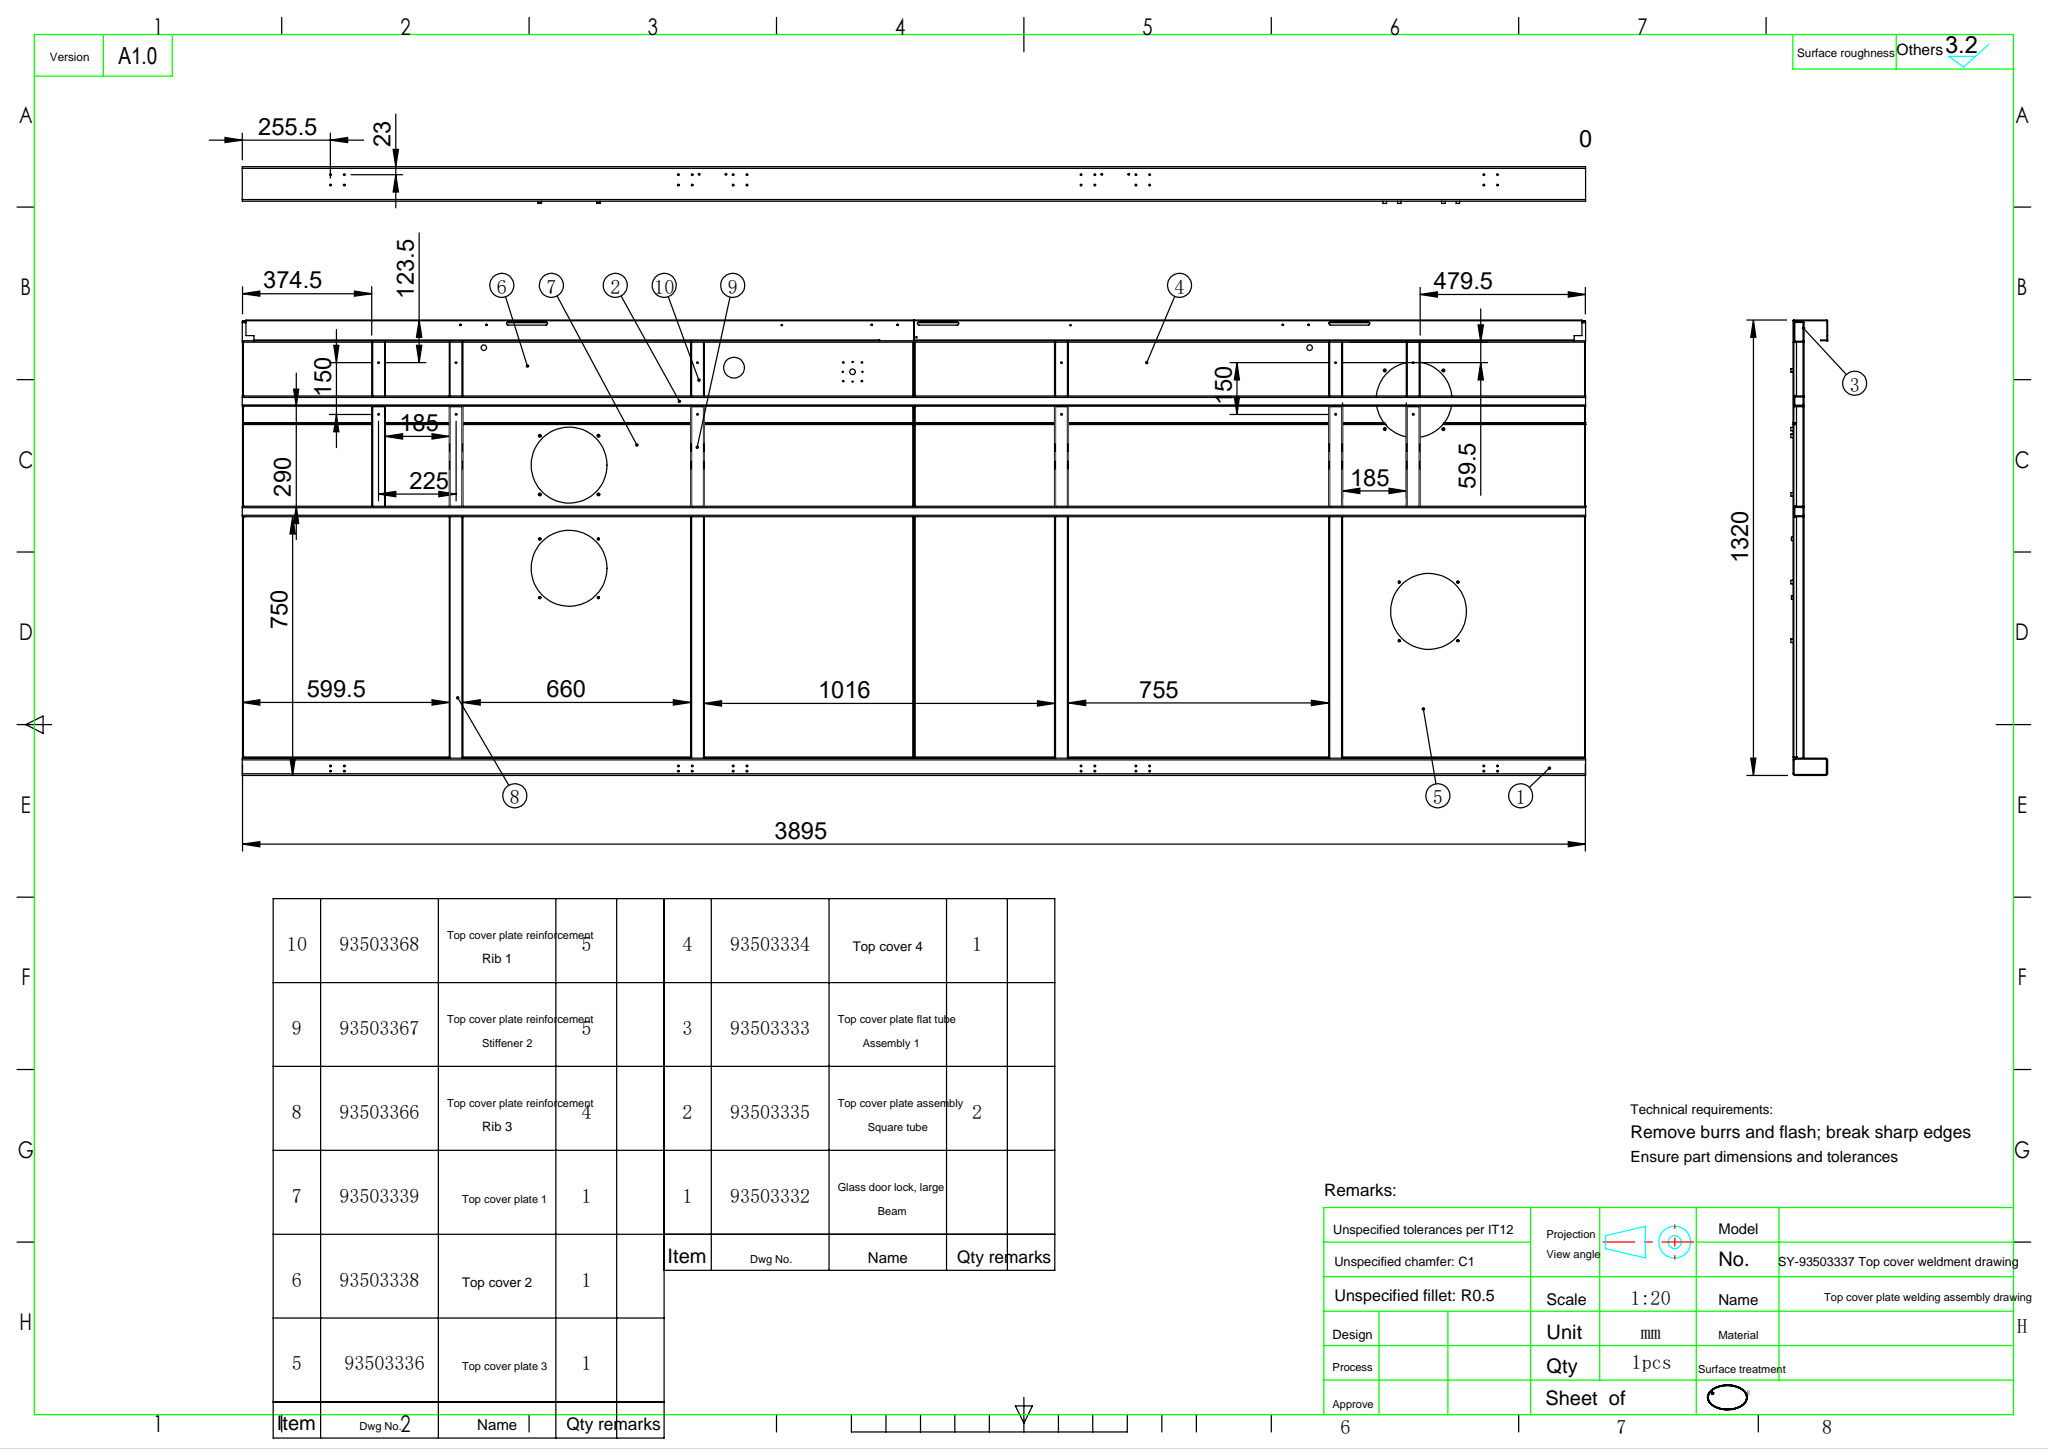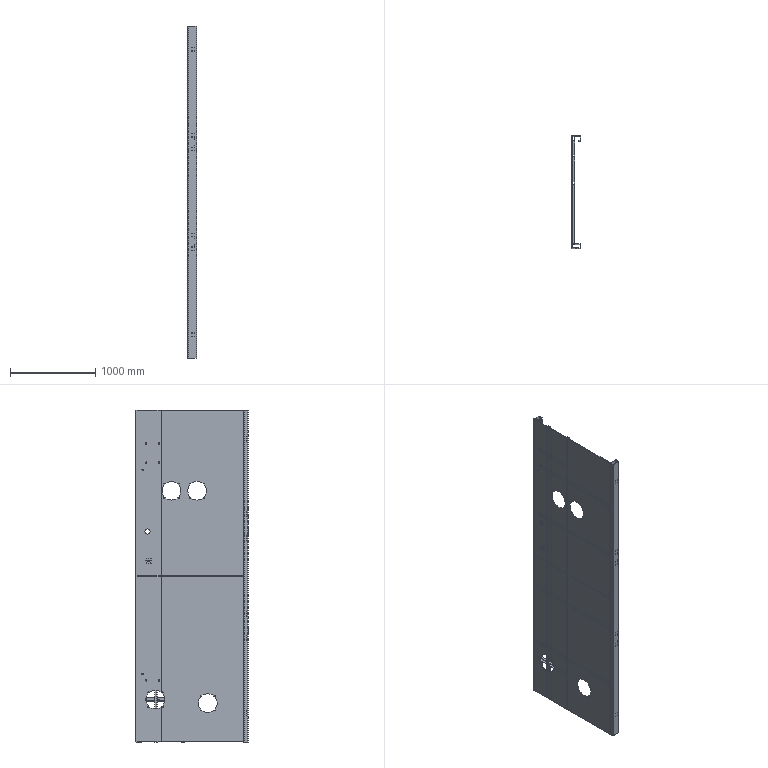Part | SolidWorks | features ReferencePattern 4, LocalLPattern 2 | 32 solids | 1226 faces | box 106 x 1320 x 3896 mm | volume 19791071 mm3 | plane 710 | cylinder 504 | cone 12 | commonest cylinder face diameters 5 x164 10 x56 4.2 x46 3.3 x42 1.473 x32 5.473 x32